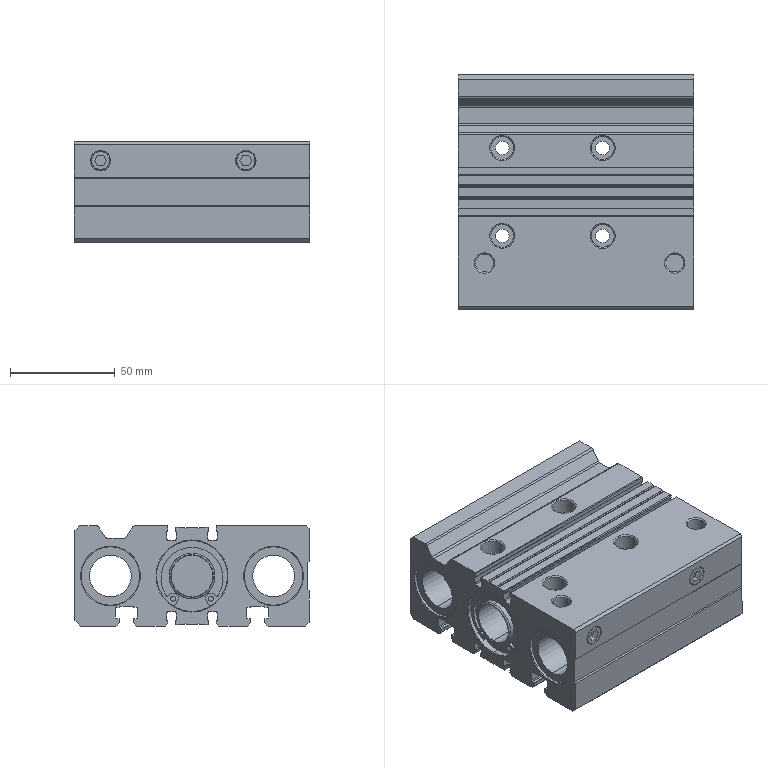Part | SolidWorks | features BaseBody 1 | 1 solid | 390 faces | box 112.5 x 112 x 48 mm | volume 379954 mm3 | cylinder 178 | plane 146 | cone 62 | spline 4 | commonest cylinder face diameters 0.4 x34 0.8 x28 6.647 x16 4 x12 1.5 x11 2.37 x8